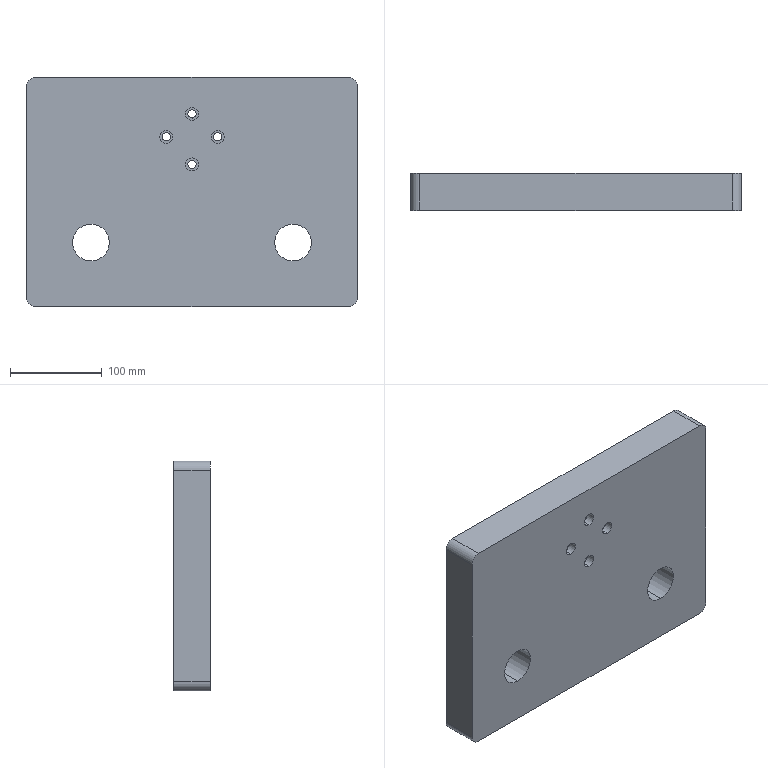Part | SolidWorks | features Extrusion 1, HoleWzd 1, ICE 1 | 1 solid | 118 faces | box 360 x 40 x 250 mm | volume 3459963 mm3 | cone 56 | cylinder 52 | plane 10 | commonest cylinder face diameters 8.5 x28 9 x8 14 x8 20 x4 40 x4